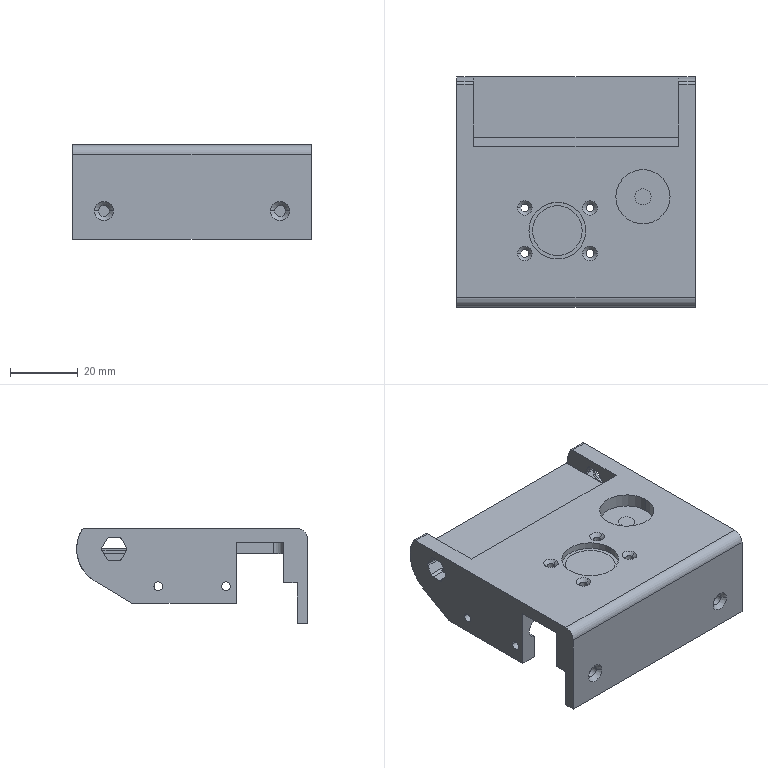NC program | NX | posted with a generic post | part box 70.5 x 68.1 x 28 mm
Lines 1 to 653 of 2864:
N10 G17 G21 G94 G90
(DRILLING_COPY_2 , TOOL : D6A45)
N12 T07 M6
N14 G54
N16 G17 G0 G90 X5. Y-5. B0. C0. S3500 M3
N18 G43 Z30. H7
N20 G94 G81 G98 Z-1. F250. R3.
N22 X57. Y-6.
N24 X50. Y-18.5
N26 G80
N28 G0 X50. Y-18.5 Z30.
N30 M5
(DRILLING_COPY_COPY_COPY_2 , TOOL : 2.5ZT)
N32 T17 M6
N34 G54
N36 G17 G0 G90 X5. Y-5. B0. C0. S2500 M3
N38 G43 Z30. H17
N40 G94 G83 G98 Z-8.5 F120. Q2. R3.
N42 G80
N44 G0 X5. Y-5. Z30.
N46 M5
(DRILLING_COPY_COPY_COPY_1_COPY , TOOL : 2.6ZT)
N48 T12 M6
N50 G54
N52 G17 G0 G90 X50. Y-18.5 B0. C0. S2500 M3
N54 G43 Z30. H12
N56 G94 G83 G98 Z-7.281 F120. Q2. R3.
N58 G80
N60 G0 X50. Y-18.5 Z30.
N62 M5
(ZLEVEL_PROFILE_COPY_COPY , TOOL : D4)
N64 T04 M6
N66 G54
N68 G17 G0 G90 X56.507 Y-4.071 B0. C0. S9500 M3
N70 G43 Z30. H4
N72 Z1.
N74 G94 G1 X56.265 Y-4.129 Z0.987 F1000.
N76 X55.786 Y-4.398 Z0.958
N78 X55.397 Y-4.787 Z0.929
N80 X55.129 Y-5.267 Z0.901
N82 X55. Y-5.801 Z0.872
N84 Y-6.201 Z0.851
N86 X55.118 Y-6.706 Z0.824
N88 X55.361 Y-7.164 Z0.796
N90 X55.713 Y-7.544 Z0.769
N92 X56.151 Y-7.822 Z0.742
N94 X56.645 Y-7.978 Z0.715
N96 X57.163 Y-8.003 Z0.688
N98 X57.67 Y-7.895 Z0.661
N100 X58.032 Y-7.725 Z0.64
N102 X58.402 Y-7.44 Z0.615
N104 X58.696 Y-7.078 Z0.591
N106 X58.899 Y-6.658 Z0.566
N108 X59. Y-6.203 Z0.542
N110 Y-5.802 Z0.521
N112 X58.9 Y-5.345 Z0.496
N114 X58.698 Y-4.924 Z0.472
N116 X58.403 Y-4.561 Z0.447
N118 X58.032 Y-4.275 Z0.423
N120 X57.67 Y-4.105 Z0.402
N122 X57.2 Y-4. Z0.377
N124 X56.8 Z0.356
N126 X56.265 Y-4.129 Z0.327
N128 X55.786 Y-4.398 Z0.298
N130 X55.397 Y-4.787 Z0.269
N132 X55.129 Y-5.267 Z0.24
N134 X55. Y-5.801 Z0.212
N136 Y-6.201 Z0.191
N138 X55.118 Y-6.706 Z0.163
N140 X55.361 Y-7.164 Z0.136
N142 X55.713 Y-7.544 Z0.109
N144 X56.151 Y-7.822 Z0.082
N146 X56.645 Y-7.978 Z0.055
N148 X57.163 Y-8.003 Z0.028
N150 X57.67 Y-7.895 Z0.
N152 X58.032 Y-7.725 Z-0.021
N154 X58.402 Y-7.44 Z-0.045
N156 X58.696 Y-7.078 Z-0.069
N158 X58.899 Y-6.658 Z-0.094
N160 X59. Y-6.203 Z-0.118
N162 Y-5.802 Z-0.139
N164 X58.9 Y-5.345 Z-0.164
N166 X58.698 Y-4.924 Z-0.188
N168 X58.403 Y-4.561 Z-0.213
N170 X58.032 Y-4.275 Z-0.237
N172 X57.67 Y-4.105 Z-0.258
N174 X57.2 Y-4. Z-0.284
N176 X57. Z-0.294
N178 G3 X55. Y-6. R2. F1300.
N180 X57. Y-4. R-2.
N182 G1 X56.862 Y-4.005 Z-0.298
N184 X56.724 Y-4.019 Z-0.303
N186 X56.587 Y-4.043 Z-0.307
N188 X56.453 Y-4.076 Z-0.311
N190 X56.321 Y-4.119 Z-0.316
N192 X56.192 Y-4.17 Z-0.32
N194 X56.067 Y-4.231 Z-0.324
N196 X55.947 Y-4.3 Z-0.329
N198 X55.832 Y-4.377 Z-0.333
N200 X55.722 Y-4.461 Z-0.337
N202 X55.619 Y-4.553 Z-0.342
N204 X55.522 Y-4.653 Z-0.346
N206 X55.432 Y-4.758 Z-0.35
N208 X55.35 Y-4.87 Z-0.355
N210 X55.276 Y-4.987 Z-0.359
N212 X55.21 Y-5.109 Z-0.363
N214 X55.152 Y-5.235 Z-0.368
N216 X55.104 Y-5.364 Z-0.372
N218 X55.064 Y-5.497 Z-0.376
N220 X55.034 Y-5.633 Z-0.381
N222 X55.013 Y-5.77 Z-0.385
N224 X55.002 Y-5.908 Z-0.389
N226 X55.001 Y-6.046 Z-0.394
N228 X55.009 Y-6.185 Z-0.398
N230 X55.026 Y-6.322 Z-0.402
N232 X55.053 Y-6.458 Z-0.407
N234 X55.09 Y-6.592 Z-0.411
N236 X55.135 Y-6.722 Z-0.415
N238 X55.19 Y-6.85 Z-0.42
N240 X55.253 Y-6.973 Z-0.424
N242 X55.324 Y-7.092 Z-0.428
N244 X55.404 Y-7.205 Z-0.433
N246 X55.491 Y-7.313 Z-0.437
N248 X55.586 Y-7.414 Z-0.441
N250 X55.687 Y-7.509 Z-0.446
N252 X55.795 Y-7.596 Z-0.45
N254 X55.908 Y-7.676 Z-0.454
N256 X56.027 Y-7.747 Z-0.458
N258 X56.15 Y-7.81 Z-0.463
N260 X56.278 Y-7.865 Z-0.467
N262 X56.408 Y-7.91 Z-0.471
N264 X56.542 Y-7.947 Z-0.476
N266 X56.678 Y-7.974 Z-0.48
N268 X56.815 Y-7.991 Z-0.484
N270 X56.954 Y-7.999 Z-0.489
N272 X57.092 Y-7.998 Z-0.493
N274 X57.23 Y-7.987 Z-0.497
N276 X57.368 Y-7.966 Z-0.502
N278 X57.503 Y-7.936 Z-0.506
N280 X57.636 Y-7.896 Z-0.51
N282 X57.765 Y-7.848 Z-0.515
N284 X57.891 Y-7.79 Z-0.519
N286 X58.013 Y-7.724 Z-0.523
N288 X58.13 Y-7.65 Z-0.528
N290 X58.242 Y-7.568 Z-0.532
N292 X58.347 Y-7.478 Z-0.536
N294 X58.447 Y-7.381 Z-0.541
N296 X58.539 Y-7.278 Z-0.545
N298 X58.623 Y-7.168 Z-0.549
N300 X58.7 Y-7.053 Z-0.554
N302 X58.769 Y-6.933 Z-0.558
N304 X58.83 Y-6.808 Z-0.562
N306 X58.881 Y-6.679 Z-0.567
N308 X58.924 Y-6.547 Z-0.571
N310 X58.957 Y-6.413 Z-0.575
N312 X58.981 Y-6.276 Z-0.58
N314 X58.995 Y-6.138 Z-0.584
N316 X59. Y-6. Z-0.588
N318 G3 X57. Y-4. R2.
N320 G1 X56.862 Y-4.005 Z-0.593
N322 X56.725 Y-4.019 Z-0.597
N324 X56.59 Y-4.043 Z-0.601
N326 X56.456 Y-4.075 Z-0.606
N328 X56.324 Y-4.118 Z-0.61
N330 X56.196 Y-4.169 Z-0.614
N332 X56.072 Y-4.228 Z-0.619
N334 X55.952 Y-4.296 Z-0.623
N336 X55.838 Y-4.372 Z-0.627
N338 X55.728 Y-4.456 Z-0.631
N340 X55.625 Y-4.548 Z-0.636
N342 X55.528 Y-4.646 Z-0.64
N344 X55.439 Y-4.75 Z-0.644
N346 X55.356 Y-4.861 Z-0.649
N348 X55.282 Y-4.977 Z-0.653
N350 X55.215 Y-5.097 Z-0.657
N352 X55.157 Y-5.222 Z-0.662
N354 X55.108 Y-5.351 Z-0.666
N356 X55.068 Y-5.483 Z-0.67
N358 X55.037 Y-5.617 Z-0.675
N360 X55.015 Y-5.753 Z-0.679
N362 X55.003 Y-5.89 Z-0.683
N364 X55. Y-6.028 Z-0.688
N366 X55.007 Y-6.166 Z-0.692
N368 X55.023 Y-6.303 Z-0.696
N370 X55.049 Y-6.438 Z-0.701
N372 X55.083 Y-6.571 Z-0.705
N374 X55.127 Y-6.702 Z-0.709
N376 X55.18 Y-6.829 Z-0.714
N378 X55.241 Y-6.953 Z-0.718
N380 X55.311 Y-7.071 Z-0.722
N382 X55.389 Y-7.185 Z-0.727
N384 X55.474 Y-7.293 Z-0.731
N386 X55.567 Y-7.395 Z-0.735
N388 X55.666 Y-7.49 Z-0.74
N390 X55.772 Y-7.579 Z-0.744
N392 X55.884 Y-7.659 Z-0.748
N394 X56.001 Y-7.732 Z-0.753
N396 X56.123 Y-7.797 Z-0.757
N398 X56.248 Y-7.853 Z-0.761
N400 X56.378 Y-7.9 Z-0.766
N402 X56.51 Y-7.938 Z-0.77
N404 X56.645 Y-7.967 Z-0.774
N406 X56.781 Y-7.987 Z-0.779
N408 X56.918 Y-7.997 Z-0.783
N410 X57.056 Y-7.998 Z-0.787
N412 X57.194 Y-7.989 Z-0.792
N414 X57.33 Y-7.971 Z-0.796
N416 X57.465 Y-7.943 Z-0.8
N418 X57.597 Y-7.906 Z-0.804
N420 X57.727 Y-7.86 Z-0.809
N422 X57.853 Y-7.805 Z-0.813
N424 X57.975 Y-7.742 Z-0.817
N426 X58.093 Y-7.67 Z-0.822
N428 X58.205 Y-7.591 Z-0.826
N430 X58.311 Y-7.504 Z-0.83
N432 X58.411 Y-7.41 Z-0.835
N434 X58.505 Y-7.309 Z-0.839
N436 X58.591 Y-7.202 Z-0.843
N438 X58.669 Y-7.089 Z-0.848
N440 X58.74 Y-6.971 Z-0.852
N442 X58.802 Y-6.849 Z-0.856
N444 X58.856 Y-6.723 Z-0.861
N446 X58.901 Y-6.593 Z-0.865
N448 X58.937 Y-6.461 Z-0.869
N450 X58.963 Y-6.326 Z-0.874
N452 X58.98 Y-6.19 Z-0.878
N454 X58.988 Y-6.053 Z-0.882
N456 G3 X57. Y-4.011 R1.989
N458 G1 X56.861 Y-4.017 Z-0.887
N460 X56.722 Y-4.032 Z-0.892
N462 X56.585 Y-4.057 Z-0.896
N464 X56.45 Y-4.092 Z-0.901
N466 X56.318 Y-4.136 Z-0.905
N468 X56.189 Y-4.189 Z-0.91
N470 X56.064 Y-4.251 Z-0.915
N472 X55.944 Y-4.322 Z-0.919
N474 X55.83 Y-4.401 Z-0.924
N476 X55.721 Y-4.488 Z-0.928
N478 X55.619 Y-4.582 Z-0.933
N480 X55.524 Y-4.683 Z-0.938
N482 X55.436 Y-4.79 Z-0.942
N484 X55.355 Y-4.903 Z-0.947
N486 X55.283 Y-5.022 Z-0.951
N488 X55.22 Y-5.145 Z-0.956
N490 X55.165 Y-5.272 Z-0.96
N492 X55.12 Y-5.403 Z-0.965
N494 X55.084 Y-5.537 Z-0.97
N496 X55.057 Y-5.673 Z-0.974
N498 X55.04 Y-5.81 Z-0.979
N500 X55.033 Y-5.948 Z-0.983
N502 X55.035 Y-6.086 Z-0.988
N504 X55.047 Y-6.223 Z-0.993
N506 X55.069 Y-6.359 Z-0.997
N508 X55.1 Y-6.494 Z-1.002
N510 X55.141 Y-6.625 Z-1.006
N512 X55.19 Y-6.754 Z-1.011
N514 X55.249 Y-6.878 Z-1.016
N516 X55.316 Y-6.998 Z-1.02
N518 X55.391 Y-7.113 Z-1.025
N520 X55.474 Y-7.222 Z-1.029
N522 X55.565 Y-7.325 Z-1.034
N524 X55.662 Y-7.421 Z-1.039
N526 X55.766 Y-7.511 Z-1.043
N528 X55.876 Y-7.592 Z-1.048
N530 X55.991 Y-7.666 Z-1.052
N532 X56.112 Y-7.731 Z-1.057
N534 X56.236 Y-7.788 Z-1.062
N536 X56.364 Y-7.835 Z-1.066
N538 X56.494 Y-7.874 Z-1.071
N540 X56.627 Y-7.903 Z-1.075
N542 X56.762 Y-7.923 Z-1.08
N544 X56.897 Y-7.933 Z-1.085
N546 X57.033 Y-7.934 Z-1.089
N548 X57.169 Y-7.925 Z-1.094
N550 X57.303 Y-7.907 Z-1.098
N552 X57.435 Y-7.879 Z-1.103
N554 X57.565 Y-7.842 Z-1.108
N556 X57.693 Y-7.796 Z-1.112
N558 X57.816 Y-7.741 Z-1.117
N560 X57.935 Y-7.678 Z-1.121
N562 X58.05 Y-7.607 Z-1.126
N564 X58.159 Y-7.528 Z-1.131
N566 X58.261 Y-7.441 Z-1.135
N568 X58.358 Y-7.348 Z-1.14
N570 X58.448 Y-7.248 Z-1.144
N572 X58.53 Y-7.142 Z-1.149
N574 X58.604 Y-7.031 Z-1.153
N576 X58.671 Y-6.914 Z-1.158
N578 X58.729 Y-6.794 Z-1.163
N580 X58.778 Y-6.67 Z-1.167
N582 X58.819 Y-6.543 Z-1.172
N584 X58.85 Y-6.414 Z-1.176
N586 G3 X57. Y-4.104 R1.896
N588 G1 X56.864 Y-4.112 Z-1.181
N590 X56.728 Y-4.129 Z-1.186
N592 X56.594 Y-4.156 Z-1.191
N594 X56.463 Y-4.192 Z-1.196
N596 X56.335 Y-4.238 Z-1.201
N598 X56.21 Y-4.293 Z-1.206
N600 X56.09 Y-4.356 Z-1.211
N602 X55.975 Y-4.429 Z-1.216
N604 X55.867 Y-4.509 Z-1.221
N606 X55.764 Y-4.597 Z-1.225
N608 X55.668 Y-4.692 Z-1.23
N610 X55.579 Y-4.794 Z-1.235
N612 X55.498 Y-4.901 Z-1.24
N614 X55.425 Y-5.014 Z-1.245
N616 X55.36 Y-5.131 Z-1.25
N618 X55.304 Y-5.253 Z-1.255
N620 X55.258 Y-5.378 Z-1.26
N622 X55.22 Y-5.507 Z-1.265
N624 X55.192 Y-5.637 Z-1.27
N626 X55.173 Y-5.769 Z-1.275
N628 X55.161 Y-5.902 Z-1.279
N630 X55.154 Y-6.034 Z-1.284
N632 X55.174 Y-6.166 Z-1.289
N634 X55.194 Y-6.297 Z-1.294
N636 X55.223 Y-6.426 Z-1.299
N638 X55.261 Y-6.553 Z-1.304
N640 X55.308 Y-6.675 Z-1.309
N642 X55.364 Y-6.795 Z-1.314
N644 X55.428 Y-6.909 Z-1.319
N646 X55.5 Y-7.019 Z-1.324
N648 X55.58 Y-7.123 Z-1.328
N650 X55.667 Y-7.22 Z-1.333
N652 X55.76 Y-7.311 Z-1.338
N654 X55.86 Y-7.395 Z-1.343
N656 X56.065 Y-7.557 Z-1.353
N658 X56.107 Y-7.584 Z-1.355
N660 X56.309 Y-7.652 Z-1.363
N662 X56.431 Y-7.695 Z-1.368
N664 X56.556 Y-7.729 Z-1.373
N666 X56.682 Y-7.753 Z-1.377
N668 X56.81 Y-7.769 Z-1.382
N670 X56.938 Y-7.775 Z-1.387
N672 X57.066 Y-7.772 Z-1.392
N674 X57.193 Y-7.76 Z-1.397
N676 X57.32 Y-7.739 Z-1.402
N678 X57.443 Y-7.708 Z-1.407
N680 X57.565 Y-7.669 Z-1.412
N682 X57.683 Y-7.622 Z-1.417
N684 X57.805 Y-7.581 Z-1.422
N686 X57.883 Y-7.557 Z-1.425
N688 X58.015 Y-7.435 Z-1.431
N690 X58.109 Y-7.352 Z-1.436
N692 X58.202 Y-7.265 Z-1.441
N694 X58.288 Y-7.173 Z-1.446
N696 X58.367 Y-7.075 Z-1.451
N698 X58.439 Y-6.973 Z-1.456
N700 X58.503 Y-6.865 Z-1.461
N702 X58.559 Y-6.753 Z-1.466
N704 X58.607 Y-6.637 Z-1.471
N706 G3 X58.703 Y-6.296 R1.728
N708 G2 X58.778 Y-5.998 R1.934
N710 G1 X58.703 Y-5.704
N712 G3 X58.108 Y-4.673 R1.728
N714 G1 X57.918 Y-4.494
N716 X57.889 Y-4.46
N718 G2 X57.595 Y-4.377 R1.441
N720 G3 X57. Y-4.272 R1.728
N722 X56.405 Y-4.377 R1.728
N724 G2 X56.111 Y-4.46 R1.466
N726 X55.892 Y-4.673 R2.338
N728 G3 X55.297 Y-5.704 R1.728
N730 G2 X55.223 Y-6. R1.824
N732 G1 X55.233 Y-6.034
N734 X55.297 Y-6.296
N736 G3 X55.869 Y-7.307 R1.728
N738 G2 X56.111 Y-7.54 R2.296
N740 X56.405 Y-7.623 R1.457
N742 G3 X57.595 Y-7.623 R1.728
N744 G1 X57.848 Y-7.549
N746 X57.889 Y-7.54
N748 X57.918 Y-7.506
N750 X58.108 Y-7.327
N752 G3 X58.607 Y-6.637 R1.728
N754 G1 Z-0.471
N756 G0 X58.184 Y-7.014
N758 G1 X58.301 Y-6.877 Z-0.48 F1000.
N760 X58.409 Y-6.688 Z-0.491
N762 X58.469 Y-6.522 Z-0.501
N764 X58.536 Y-6.336 Z-0.511
N766 X58.636 Y-6.166 Z-0.521
N768 X58.732 Y-6. Z-0.531
N770 X58.637 Y-5.835 Z-0.541
N772 X58.536 Y-5.664 Z-0.552
N774 X58.469 Y-5.478 Z-0.562
N776 X58.409 Y-5.312 Z-0.571
N778 X58.214 Y-5.007 Z-0.59
N780 X58.088 Y-4.884 Z-0.6
N782 X57.866 Y-4.5 Z-0.623
N784 X57.65 Z-0.634
N786 X57.283 Y-4.467 Z-0.654
N788 X57.142 Y-4.442 Z-0.661
N790 X56.858 Z-0.676
N792 X56.717 Y-4.467 Z-0.683
N794 X56.35 Y-4.5 Z-0.703
N796 X56.134 Z-0.714
N798 X56.01 Y-4.714 Z-0.727
N800 X55.814 Y-4.989 Z-0.745
N802 X55.699 Y-5.123 Z-0.754
N804 X55.591 Y-5.312 Z-0.765
N806 X55.531 Y-5.478 Z-0.775
N808 X55.463 Y-5.665 Z-0.785
N810 X55.363 Y-5.836 Z-0.795
N812 X55.268 Y-6. Z-0.805
N814 X55.489 Y-6.384 Z-0.829
N816 X55.533 Y-6.555 Z-0.838
N818 X55.699 Y-6.876 Z-0.857
N820 X55.814 Y-7.011 Z-0.866
N822 X56.01 Y-7.286 Z-0.884
N824 X56.134 Y-7.5 Z-0.897
N826 X56.329 Z-0.907
N828 X56.525 Y-7.499 Z-0.917
N830 X56.717 Y-7.533 Z-0.928
N832 X56.891 Y-7.565 Z-0.937
N834 X57.109 Z-0.948
N836 X57.283 Y-7.533 Z-0.957
N838 X57.476 Y-7.499 Z-0.968
N840 X57.671 Y-7.5 Z-0.978
N842 X57.866 Z-0.988
N844 X57.981 Y-7.301 Z-1.
N846 X58.07 Y-7.147 Z-1.01
N848 X58.186 Y-7.011 Z-1.019
N850 X58.301 Y-6.877 Z-1.028
N852 X58.409 Y-6.688 Z-1.04
N854 X58.469 Y-6.522 Z-1.049
N856 X58.536 Y-6.336 Z-1.059
N858 X58.636 Y-6.166 Z-1.07
N860 X58.732 Y-6. Z-1.08
N862 X58.637 Y-5.835 Z-1.09
N864 X58.536 Y-5.664 Z-1.1
N866 X58.469 Y-5.478 Z-1.11
N868 X58.409 Y-5.312 Z-1.12
N870 X58.214 Y-5.007 Z-1.139
N872 X58.088 Y-4.884 Z-1.148
N874 X57.866 Y-4.5 Z-1.171
N876 X57.65 Z-1.182
N878 X57.283 Y-4.467 Z-1.202
N880 X57.142 Y-4.442 Z-1.209
N882 X56.858 Z-1.224
N884 X56.717 Y-4.467 Z-1.232
N886 X56.35 Y-4.5 Z-1.251
N888 X56.134 Z-1.262
N890 X56.01 Y-4.714 Z-1.275
N892 X55.814 Y-4.989 Z-1.293
N894 X55.699 Y-5.123 Z-1.302
N896 X55.591 Y-5.312 Z-1.314
N898 X55.531 Y-5.478 Z-1.323
N900 X55.463 Y-5.665 Z-1.333
N902 X55.363 Y-5.836 Z-1.344
N904 X55.268 Y-6. Z-1.354
N906 X55.489 Y-6.384 Z-1.377
N908 X55.533 Y-6.555 Z-1.386
N910 X55.699 Y-6.876 Z-1.405
N912 X55.814 Y-7.011 Z-1.414
N914 X56.01 Y-7.286 Z-1.432
N916 X56.134 Y-7.5 Z-1.445
N918 X56.329 Z-1.455
N920 X56.525 Y-7.499 Z-1.465
N922 X56.717 Y-7.533 Z-1.476
N924 X56.891 Y-7.565 Z-1.485
N926 X57.109 Z-1.496
N928 X57.283 Y-7.533 Z-1.506
N930 X57.476 Y-7.499 Z-1.516
N932 X57.671 Y-7.5 Z-1.526
N934 X57.866 Z-1.536
N936 X57.981 Y-7.301 Z-1.548
N938 X58.07 Y-7.147 Z-1.558
N940 X58.186 Y-7.011 Z-1.567
N942 X58.301 Y-6.877 Z-1.576
N944 X58.409 Y-6.688 Z-1.588
N946 X58.469 Y-6.522 Z-1.597
N948 X58.536 Y-6.336 Z-1.607
N950 X58.636 Y-6.166 Z-1.618
N952 X58.732 Y-6. Z-1.628
N954 X58.637 Y-5.835 Z-1.638
N956 X58.536 Y-5.664 Z-1.648
N958 X58.469 Y-5.478 Z-1.658
N960 X58.409 Y-5.312 Z-1.668
N962 X58.214 Y-5.007 Z-1.687
N964 X58.088 Y-4.884 Z-1.696
N966 X57.866 Y-4.5 Z-1.719
N968 X57.65 Z-1.73
N970 X57.283 Y-4.467 Z-1.75
N972 X57.142 Y-4.442 Z-1.757
N974 X57. Z-1.765
N976 G3 X56.717 Y-4.467 R1.558 F1300.
N978 G1 X56.35 Y-4.5
N980 X56.134
N982 X56.01 Y-4.714
N984 X55.814 Y-4.989
N986 G3 X55.531 Y-5.478 R1.558
N988 G2 X55.363 Y-5.836 R2.17
N990 G1 X55.268 Y-6.
N992 X55.489 Y-6.384
N994 G3 X55.814 Y-7.011 R1.558
N996 G1 X56.01 Y-7.286
N998 X56.134 Y-7.5
N1000 X56.329
N1002 G2 X56.717 Y-7.533 R2.142
N1004 G3 X57.283 Y-7.533 R1.558
N1006 G2 X57.671 Y-7.5 R2.143
N1008 G1 X57.866
N1010 X57.981 Y-7.301
N1012 G2 X58.186 Y-7.011 R1.95
N1014 G3 X58.469 Y-6.522 R1.558
N1016 G2 X58.636 Y-6.166 R2.16
N1018 G1 X58.732 Y-6.
N1020 X58.637 Y-5.835
N1022 G2 X58.469 Y-5.478 R2.163
N1024 G3 X58.088 Y-4.884 R1.558
N1026 G1 X57.866 Y-4.5
N1028 X57.65
N1030 X57.283 Y-4.467
N1032 G3 X57. Y-4.442 R1.558
N1034 G1 X56.862 Y-4.451 Z-1.77
N1036 X56.724 Y-4.472 Z-1.775
N1038 X56.586 Y-4.488 Z-1.78
N1040 X56.447 Y-4.5 Z-1.786
N1042 X56.307 Z-1.791
N1044 X56.14 Z-1.797
N1046 X56.012 Y-4.712 Z-1.807
N1048 X55.942 Y-4.833 Z-1.812
N1050 X55.867 Y-4.951 Z-1.817
N1052 X55.792 Y-5.066 Z-1.822
N1054 X55.716 Y-5.182 Z-1.828
N1056 X55.651 Y-5.301 Z-1.833
N1058 X55.594 Y-5.424 Z-1.838
N1060 X55.529 Y-5.548 Z-1.843
N1062 X55.459 Y-5.67 Z-1.849
N1064 X55.319 Y-5.911 Z-1.859
N1066 X55.268 Y-6. Z-1.863
N1068 X55.356 Y-6.152 Z-1.87
N1070 X55.495 Y-6.394 Z-1.88
N1072 X55.634 Y-6.634 Z-1.891
N1074 X55.768 Y-6.867 Z-1.901
N1076 X55.908 Y-7.108 Z-1.912
N1078 X56.048 Y-7.35 Z-1.922
N1080 X56.134 Y-7.5 Z-1.929
N1082 X56.24 Z-1.933
N1084 X56.518 Z-1.943
N1086 X56.799 Z-1.954
N1088 X57.069 Z-1.964
N1090 X57.344 Z-1.975
N1092 X57.624 Z-1.985
N1094 X57.866 Z-1.994
N1096 X57.884 Y-7.468 Z-1.996
N1098 X58.024 Y-7.227 Z-2.006
N1100 X58.165 Y-6.983 Z-2.017
N1102 X58.3 Y-6.748 Z-2.027
N1104 X58.436 Y-6.514 Z-2.038
N1106 X58.577 Y-6.269 Z-2.048
N1108 X58.716 Y-6.028 Z-2.059
N1110 X58.732 Y-6.
N1112 X57.866 Y-4.5
N1114 X57.
N1116 X56.134 Z-2.092
N1118 X55.268 Y-6. Z-2.157
N1120 X56.134 Y-7.5 Z-2.222
N1122 X57.866 Z-2.288
N1124 X58.732 Y-6. Z-2.353
N1126 X57.866 Y-4.5
N1128 X57.
N1130 X56.134 Z-2.386
N1132 X55.268 Y-6. Z-2.451
N1134 X56.134 Y-7.5 Z-2.516
N1136 X57.866 Z-2.582
N1138 X58.732 Y-6. Z-2.647
N1140 X57.866 Y-4.5
N1142 X57.
N1144 X56.134 Z-2.68
N1146 X55.268 Y-6. Z-2.745
N1148 X56.134 Y-7.5 Z-2.81
N1150 X57.866 Z-2.876
N1152 X58.732 Y-6. Z-2.941
N1154 X57.866 Y-4.5
N1156 X57.
N1158 X56.134 Z-2.974
N1160 X55.268 Y-6. Z-3.039
N1162 X56.134 Y-7.5 Z-3.105
N1164 X57.866 Z-3.17
N1166 X58.732 Y-6. Z-3.235
N1168 X57.866 Y-4.5
N1170 X57.
N1172 X56.134 Z-3.268
N1174 X55.268 Y-6. Z-3.333
N1176 X56.134 Y-7.5 Z-3.399
N1178 X57.866 Z-3.464
N1180 X58.732 Y-6. Z-3.529
N1182 X57.866 Y-4.5
N1184 X57.
N1186 X56.134 Z-3.562
N1188 X55.268 Y-6. Z-3.627
N1190 X56.134 Y-7.5 Z-3.693
N1192 X57.866 Z-3.758
N1194 X58.732 Y-6. Z-3.824
N1196 X57.866 Y-4.5
N1198 X57.
N1200 X56.134 Z-3.856
N1202 X55.268 Y-6. Z-3.922
N1204 X56.134 Y-7.5 Z-3.987
N1206 X57.866 Z-4.052
N1208 X58.732 Y-6. Z-4.118
N1210 X57.866 Y-4.5
N1212 X57.
N1214 X56.134 Z-4.15
N1216 X55.268 Y-6. Z-4.216
N1218 X56.134 Y-7.5 Z-4.281
N1220 X57.866 Z-4.346
N1222 X58.732 Y-6. Z-4.412
N1224 X57.866 Y-4.5
N1226 X57.
N1228 X56.134 Z-4.444
N1230 X55.268 Y-6. Z-4.51
N1232 X56.057 Y-7.366 Z-4.569
N1234 X56.134 Y-7.5 Z-4.575
N1236 X56.258 Z-4.58
N1238 X57.866 Z-4.641
N1240 X58.732 Y-6. Z-4.706
N1242 X57.866 Y-4.5
N1244 X57.
N1246 X56.134 Z-4.739
N1248 X55.268 Y-6. Z-4.804
N1250 X56.057 Y-7.366 Z-4.863
N1252 X56.133 Y-7.499 Z-4.869
N1254 X56.258 Z-4.874
N1256 X56.397 Y-7.5 Z-4.879
N1258 X57.371 Z-4.916
N1260 X57.51 Y-7.499 Z-4.921
N1262 X57.65 Z-4.926
N1264 X57.867 Z-4.935
N1266 X57.897 Y-7.446 Z-4.937
N1268 X58.732 Y-6. Z-5.
N1270 X57.866 Y-4.5
N1272 X56.134
N1274 X55.268 Y-6.
N1276 X56.134 Y-7.5
N1278 X57.866
N1280 X58.732 Y-6.
N1282 Z-4.
N1284 G0 Z30.
N1286 M5